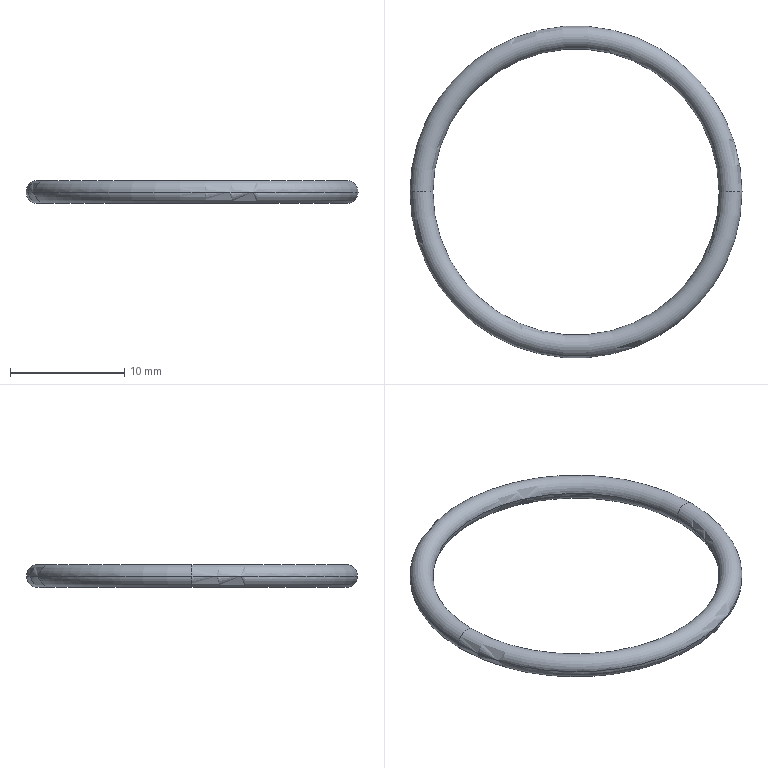Part | SolidWorks | features RefAxis 1, Revolution 1 | 1 solid | 4 faces | box 29 x 29 x 2 mm | volume 266.479 mm3 | torus 4
STEP:
#1=CARTESIAN_POINT('',(14.5,0.,0.));
#2=VERTEX_POINT('',#1);
#3=CARTESIAN_POINT('',(12.5,0.,0.));
#4=VERTEX_POINT('',#3);
#5=CARTESIAN_POINT('',(13.5,0.,0.));
#6=DIRECTION('',(0.,1.,0.));
#7=DIRECTION('',(-1.,0.,0.));
#8=AXIS2_PLACEMENT_3D('',#5,#6,#7);
#9=CIRCLE('',#8,1.);
#10=EDGE_CURVE('',#2,#4,#9,.T.);
#11=ORIENTED_EDGE('',*,*,#10,.F.);
#12=CARTESIAN_POINT('',(-14.5,0.,0.));
#13=VERTEX_POINT('',#12);
#14=CARTESIAN_POINT('',(0.,0.,0.));
#15=DIRECTION('',(0.,0.,-1.));
#16=DIRECTION('',(-1.,0.,0.));
#17=AXIS2_PLACEMENT_3D('',#14,#15,#16);
#18=CIRCLE('',#17,14.5);
#19=EDGE_CURVE('',#2,#13,#18,.T.);
#20=ORIENTED_EDGE('',*,*,#19,.T.);
#21=CARTESIAN_POINT('',(-12.5,0.,0.));
#22=VERTEX_POINT('',#21);
#23=CARTESIAN_POINT('',(-13.5,0.,0.));
#24=DIRECTION('',(0.,-1.,0.));
#25=DIRECTION('',(0.,0.,-1.));
#26=AXIS2_PLACEMENT_3D('',#23,#24,#25);
#27=CIRCLE('',#26,1.);
#28=EDGE_CURVE('',#13,#22,#27,.T.);
#29=ORIENTED_EDGE('',*,*,#28,.T.);
#30=CARTESIAN_POINT('',(0.,0.,0.));
#31=DIRECTION('',(0.,0.,-1.));
#32=DIRECTION('',(-1.,0.,0.));
#33=AXIS2_PLACEMENT_3D('',#30,#31,#32);
#34=CIRCLE('',#33,12.5);
#35=EDGE_CURVE('',#4,#22,#34,.T.);
#36=ORIENTED_EDGE('',*,*,#35,.F.);
#37=EDGE_LOOP('',(#11,#20,#29,#36));
#38=FACE_OUTER_BOUND('',#37,.T.);
#39=CARTESIAN_POINT('',(0.,0.,0.));
#40=DIRECTION('',(0.,0.,-1.));
#41=DIRECTION('',(-1.,0.,0.));
#42=AXIS2_PLACEMENT_3D('',#39,#40,#41);
#43=TOROIDAL_SURFACE('',#42,13.5,1.);
#44=ADVANCED_FACE('',(#38),#43,.T.);
#45=ORIENTED_EDGE('',*,*,#28,.F.);
#46=CARTESIAN_POINT('',(0.,0.,0.));
#47=DIRECTION('',(0.,0.,-1.));
#48=DIRECTION('',(-1.,0.,0.));
#49=AXIS2_PLACEMENT_3D('',#46,#47,#48);
#50=CIRCLE('',#49,14.5);
#51=EDGE_CURVE('',#13,#2,#50,.T.);
#52=ORIENTED_EDGE('',*,*,#51,.T.);
#53=ORIENTED_EDGE('',*,*,#10,.T.);
#54=CARTESIAN_POINT('',(0.,0.,0.));
#55=DIRECTION('',(0.,0.,-1.));
#56=DIRECTION('',(-1.,0.,0.));
#57=AXIS2_PLACEMENT_3D('',#54,#55,#56);
#58=CIRCLE('',#57,12.5);
#59=EDGE_CURVE('',#22,#4,#58,.T.);
#60=ORIENTED_EDGE('',*,*,#59,.F.);
#61=EDGE_LOOP('',(#45,#52,#53,#60));
#62=FACE_OUTER_BOUND('',#61,.T.);
#63=CARTESIAN_POINT('',(0.,0.,0.));
#64=DIRECTION('',(0.,0.,-1.));
#65=DIRECTION('',(-1.,0.,0.));
#66=AXIS2_PLACEMENT_3D('',#63,#64,#65);
#67=TOROIDAL_SURFACE('',#66,13.5,1.);
#68=ADVANCED_FACE('',(#62),#67,.T.);
#69=ORIENTED_EDGE('',*,*,#51,.F.);
#70=CARTESIAN_POINT('',(-13.5,0.,0.));
#71=DIRECTION('',(0.,-1.,0.));
#72=DIRECTION('',(0.,0.,-1.));
#73=AXIS2_PLACEMENT_3D('',#70,#71,#72);
#74=CIRCLE('',#73,1.);
#75=EDGE_CURVE('',#22,#13,#74,.T.);
#76=ORIENTED_EDGE('',*,*,#75,.F.);
#77=ORIENTED_EDGE('',*,*,#59,.T.);
#78=CARTESIAN_POINT('',(13.5,0.,0.));
#79=DIRECTION('',(0.,1.,0.));
#80=DIRECTION('',(-1.,0.,0.));
#81=AXIS2_PLACEMENT_3D('',#78,#79,#80);
#82=CIRCLE('',#81,1.);
#83=EDGE_CURVE('',#4,#2,#82,.T.);
#84=ORIENTED_EDGE('',*,*,#83,.T.);
#85=EDGE_LOOP('',(#69,#76,#77,#84));
#86=FACE_OUTER_BOUND('',#85,.T.);
#87=CARTESIAN_POINT('',(0.,0.,0.));
#88=DIRECTION('',(0.,0.,-1.));
#89=DIRECTION('',(-1.,0.,0.));
#90=AXIS2_PLACEMENT_3D('',#87,#88,#89);
#91=TOROIDAL_SURFACE('',#90,13.5,1.);
#92=ADVANCED_FACE('',(#86),#91,.T.);
#93=ORIENTED_EDGE('',*,*,#19,.F.);
#94=ORIENTED_EDGE('',*,*,#83,.F.);
#95=ORIENTED_EDGE('',*,*,#35,.T.);
#96=ORIENTED_EDGE('',*,*,#75,.T.);
#97=EDGE_LOOP('',(#93,#94,#95,#96));
#98=FACE_OUTER_BOUND('',#97,.T.);
#99=CARTESIAN_POINT('',(0.,0.,0.));
#100=DIRECTION('',(0.,0.,-1.));
#101=DIRECTION('',(-1.,0.,0.));
#102=AXIS2_PLACEMENT_3D('',#99,#100,#101);
#103=TOROIDAL_SURFACE('',#102,13.5,1.);
#104=ADVANCED_FACE('',(#98),#103,.T.);
#105=CLOSED_SHELL('',(#44,#68,#92,#104));
#106=MANIFOLD_SOLID_BREP('',#105);
#107=CARTESIAN_POINT('',(0.,0.,0.));
#108=DIRECTION('',(0.,0.,1.));
#109=DIRECTION('',(1.,0.,0.));
#110=AXIS2_PLACEMENT_3D('',#107,#108,#109);
#111=(LENGTH_UNIT()NAMED_UNIT(*)SI_UNIT(.MILLI.,.METRE.));
#112=UNCERTAINTY_MEASURE_WITH_UNIT(LENGTH_MEASURE(0.00001),#111,'','');
#113=(NAMED_UNIT(*)PLANE_ANGLE_UNIT()SI_UNIT($,.RADIAN.));
#114=(NAMED_UNIT(*)SI_UNIT($,.STERADIAN.)SOLID_ANGLE_UNIT());
#115=(GEOMETRIC_REPRESENTATION_CONTEXT(3)GLOBAL_UNCERTAINTY_ASSIGNED_CONTEXT((#112))GLOBAL_UNIT_ASSIGNED_CONTEXT((#111,#113,#114))REPRESENTATION_CONTEXT('',''));
#116=ADVANCED_BREP_SHAPE_REPRESENTATION('',(#106,#110),#115);